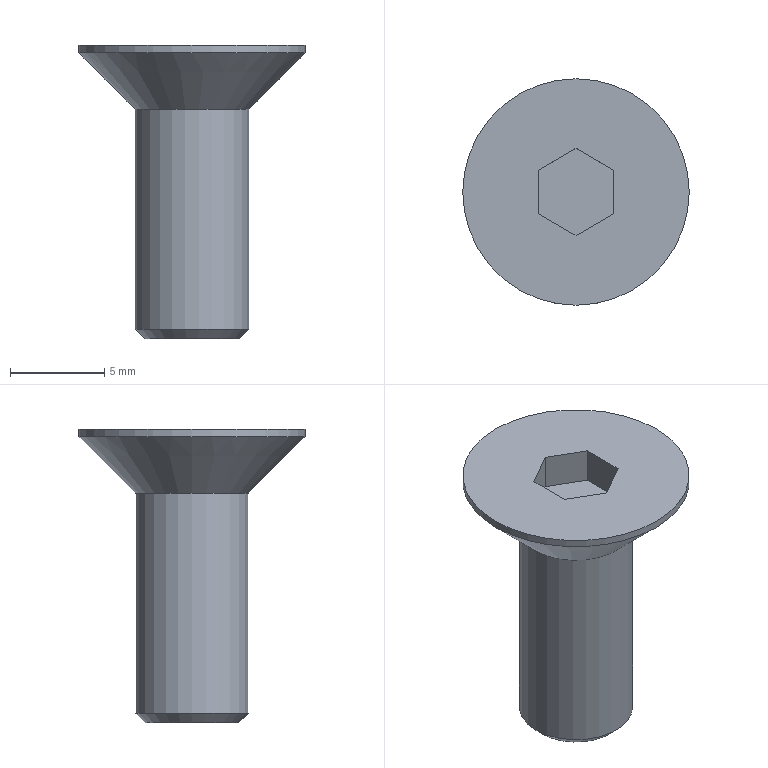Part | STEP file | solid 154 | 1 solid | 13 faces | box 12 x 12 x 15.55 mm | volume 558.14 mm3 | plane 9 | cone 2 | cylinder 2 | commonest cylinder face diameters 6 x1 12 x1